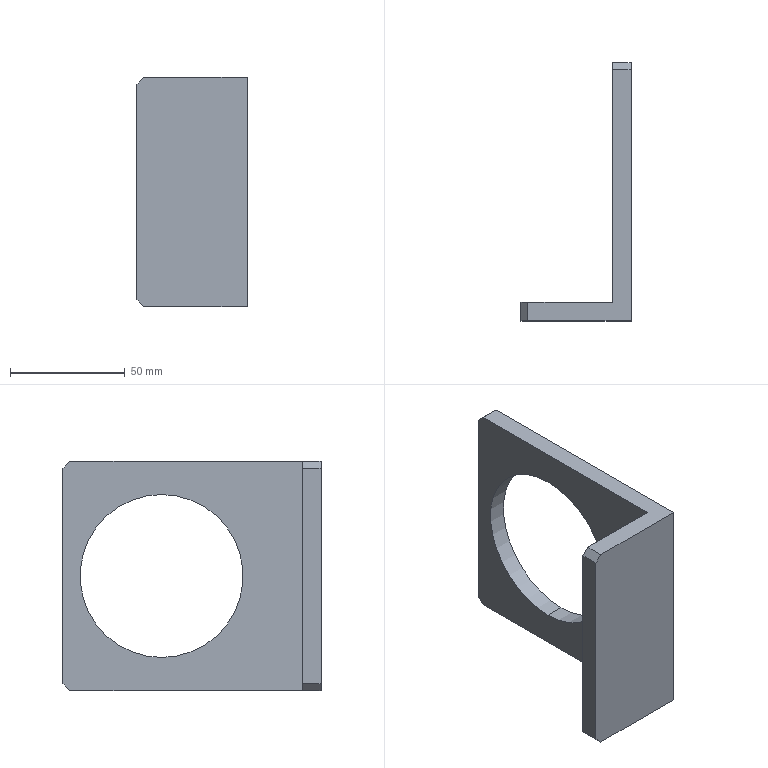Part | SolidWorks | features Chamfer 1, Extrusion 1, ICE 1 | 1 solid | 14 faces | box 48 x 112.5 x 100 mm | volume 90182 mm3 | plane 12 | cylinder 2 | commonest cylinder face diameters 71 x2
STEP:
#1=CARTESIAN_POINT('',(0.,69.5,1.121));
#2=VERTEX_POINT('',#1);
#3=CARTESIAN_POINT('',(0.,69.5,-69.879));
#4=VERTEX_POINT('',#3);
#5=CARTESIAN_POINT('',(0.,69.5,-34.379));
#6=DIRECTION('',(1.,0.,0.));
#7=DIRECTION('',(0.,0.,1.));
#8=AXIS2_PLACEMENT_3D('',#5,#6,#7);
#9=CIRCLE('',#8,35.5);
#10=EDGE_CURVE('',#2,#4,#9,.T.);
#11=ORIENTED_EDGE('',*,*,#10,.T.);
#12=CARTESIAN_POINT('',(-8.,69.5,-69.879));
#13=VERTEX_POINT('',#12);
#14=CARTESIAN_POINT('',(0.001,69.5,-69.879));
#15=DIRECTION('',(-1.,0.,0.));
#16=VECTOR('',#15,1000.);
#17=LINE('',#14,#16);
#18=EDGE_CURVE('',#4,#13,#17,.T.);
#19=ORIENTED_EDGE('',*,*,#18,.T.);
#20=CARTESIAN_POINT('',(-8.,69.5,1.121));
#21=VERTEX_POINT('',#20);
#22=CARTESIAN_POINT('',(-8.,69.5,-34.379));
#23=DIRECTION('',(-1.,0.,0.));
#24=DIRECTION('',(0.,0.,1.));
#25=AXIS2_PLACEMENT_3D('',#22,#23,#24);
#26=CIRCLE('',#25,35.5);
#27=EDGE_CURVE('',#13,#21,#26,.T.);
#28=ORIENTED_EDGE('',*,*,#27,.T.);
#29=CARTESIAN_POINT('',(0.001,69.5,1.121));
#30=DIRECTION('',(-1.,0.,0.));
#31=VECTOR('',#30,1000.);
#32=LINE('',#29,#31);
#33=EDGE_CURVE('',#2,#21,#32,.T.);
#34=ORIENTED_EDGE('',*,*,#33,.F.);
#35=EDGE_LOOP('',(#11,#19,#28,#34));
#36=FACE_OUTER_BOUND('',#35,.T.);
#37=CARTESIAN_POINT('',(0.001,69.5,-34.379));
#38=DIRECTION('',(-1.,0.,0.));
#39=DIRECTION('',(0.,0.,1.));
#40=AXIS2_PLACEMENT_3D('',#37,#38,#39);
#41=CYLINDRICAL_SURFACE('',#40,35.5);
#42=ADVANCED_FACE('',(#36),#41,.F.);
#43=CARTESIAN_POINT('',(-8.,112.5,12.621));
#44=VERTEX_POINT('',#43);
#45=CARTESIAN_POINT('',(-8.,112.5,-81.379));
#46=VERTEX_POINT('',#45);
#47=CARTESIAN_POINT('',(-8.,112.5,15.621));
#48=DIRECTION('',(0.,0.,-1.));
#49=VECTOR('',#48,1000.);
#50=LINE('',#47,#49);
#51=EDGE_CURVE('',#44,#46,#50,.T.);
#52=ORIENTED_EDGE('',*,*,#51,.F.);
#53=CARTESIAN_POINT('',(0.,112.5,12.621));
#54=VERTEX_POINT('',#53);
#55=CARTESIAN_POINT('',(-8.,112.5,12.621));
#56=DIRECTION('',(1.,0.,0.));
#57=VECTOR('',#56,1000.);
#58=LINE('',#55,#57);
#59=EDGE_CURVE('',#44,#54,#58,.T.);
#60=ORIENTED_EDGE('',*,*,#59,.T.);
#61=CARTESIAN_POINT('',(0.,112.5,-81.379));
#62=VERTEX_POINT('',#61);
#63=CARTESIAN_POINT('',(0.,112.5,15.621));
#64=DIRECTION('',(0.,0.,-1.));
#65=VECTOR('',#64,1000.);
#66=LINE('',#63,#65);
#67=EDGE_CURVE('',#54,#62,#66,.T.);
#68=ORIENTED_EDGE('',*,*,#67,.T.);
#69=CARTESIAN_POINT('',(-8.,112.5,-81.379));
#70=DIRECTION('',(-1.,0.,0.));
#71=VECTOR('',#70,1000.);
#72=LINE('',#69,#71);
#73=EDGE_CURVE('',#62,#46,#72,.T.);
#74=ORIENTED_EDGE('',*,*,#73,.T.);
#75=EDGE_LOOP('',(#52,#60,#68,#74));
#76=FACE_OUTER_BOUND('',#75,.T.);
#77=CARTESIAN_POINT('',(-8.,112.5,15.621));
#78=DIRECTION('',(0.,-1.,0.));
#79=DIRECTION('',(0.,0.,-1.));
#80=AXIS2_PLACEMENT_3D('',#77,#78,#79);
#81=PLANE('',#80);
#82=ADVANCED_FACE('',(#76),#81,.F.);
#83=CARTESIAN_POINT('',(-8.,69.5,-34.379));
#84=DIRECTION('',(-1.,0.,0.));
#85=DIRECTION('',(0.,0.,1.));
#86=AXIS2_PLACEMENT_3D('',#83,#84,#85);
#87=CIRCLE('',#86,35.5);
#88=EDGE_CURVE('',#21,#13,#87,.T.);
#89=ORIENTED_EDGE('',*,*,#88,.F.);
#90=ORIENTED_EDGE('',*,*,#27,.F.);
#91=EDGE_LOOP('',(#89,#90));
#92=FACE_BOUND('',#91,.T.);
#93=CARTESIAN_POINT('',(-8.,109.5,15.621));
#94=VERTEX_POINT('',#93);
#95=CARTESIAN_POINT('',(-8.,8.,15.621));
#96=VERTEX_POINT('',#95);
#97=CARTESIAN_POINT('',(-8.,8.,15.621));
#98=DIRECTION('',(0.,-1.,0.));
#99=VECTOR('',#98,1000.);
#100=LINE('',#97,#99);
#101=EDGE_CURVE('',#94,#96,#100,.T.);
#102=ORIENTED_EDGE('',*,*,#101,.F.);
#103=CARTESIAN_POINT('',(-8.,109.5,15.621));
#104=DIRECTION('',(0.,0.7071,-0.7071));
#105=VECTOR('',#104,1000.);
#106=LINE('',#103,#105);
#107=EDGE_CURVE('',#94,#44,#106,.T.);
#108=ORIENTED_EDGE('',*,*,#107,.T.);
#109=ORIENTED_EDGE('',*,*,#51,.T.);
#110=CARTESIAN_POINT('',(-8.,109.5,-84.379));
#111=VERTEX_POINT('',#110);
#112=CARTESIAN_POINT('',(-8.,112.5,-81.379));
#113=DIRECTION('',(0.,-0.7071,-0.7071));
#114=VECTOR('',#113,1000.);
#115=LINE('',#112,#114);
#116=EDGE_CURVE('',#46,#111,#115,.T.);
#117=ORIENTED_EDGE('',*,*,#116,.T.);
#118=CARTESIAN_POINT('',(-8.,8.,-84.379));
#119=VERTEX_POINT('',#118);
#120=CARTESIAN_POINT('',(-8.,8.,-84.379));
#121=DIRECTION('',(0.,-1.,0.));
#122=VECTOR('',#121,1000.);
#123=LINE('',#120,#122);
#124=EDGE_CURVE('',#111,#119,#123,.T.);
#125=ORIENTED_EDGE('',*,*,#124,.T.);
#126=CARTESIAN_POINT('',(-8.,8.,15.621));
#127=DIRECTION('',(0.,0.,-1.));
#128=VECTOR('',#127,1000.);
#129=LINE('',#126,#128);
#130=EDGE_CURVE('',#96,#119,#129,.T.);
#131=ORIENTED_EDGE('',*,*,#130,.F.);
#132=EDGE_LOOP('',(#102,#108,#109,#117,#125,#131));
#133=FACE_OUTER_BOUND('',#132,.T.);
#134=CARTESIAN_POINT('',(-8.,8.,15.621));
#135=DIRECTION('',(1.,0.,0.));
#136=DIRECTION('',(0.,0.,-1.));
#137=AXIS2_PLACEMENT_3D('',#134,#135,#136);
#138=PLANE('',#137);
#139=ADVANCED_FACE('',(#92,#133),#138,.F.);
#140=CARTESIAN_POINT('',(-45.,8.,-84.379));
#141=VERTEX_POINT('',#140);
#142=CARTESIAN_POINT('',(-48.,8.,-84.379));
#143=DIRECTION('',(-1.,0.,0.));
#144=VECTOR('',#143,1000.);
#145=LINE('',#142,#144);
#146=EDGE_CURVE('',#119,#141,#145,.T.);
#147=ORIENTED_EDGE('',*,*,#146,.T.);
#148=CARTESIAN_POINT('',(-48.,8.,-81.379));
#149=VERTEX_POINT('',#148);
#150=CARTESIAN_POINT('',(-48.,8.,-81.379));
#151=DIRECTION('',(-0.7071,0.,0.7071));
#152=VECTOR('',#151,1000.);
#153=LINE('',#150,#152);
#154=EDGE_CURVE('',#141,#149,#153,.T.);
#155=ORIENTED_EDGE('',*,*,#154,.T.);
#156=CARTESIAN_POINT('',(-48.,8.,12.621));
#157=VERTEX_POINT('',#156);
#158=CARTESIAN_POINT('',(-48.,8.,15.621));
#159=DIRECTION('',(0.,0.,-1.));
#160=VECTOR('',#159,1000.);
#161=LINE('',#158,#160);
#162=EDGE_CURVE('',#157,#149,#161,.T.);
#163=ORIENTED_EDGE('',*,*,#162,.F.);
#164=CARTESIAN_POINT('',(-45.,8.,15.621));
#165=VERTEX_POINT('',#164);
#166=CARTESIAN_POINT('',(-45.,8.,15.621));
#167=DIRECTION('',(0.7071,0.,0.7071));
#168=VECTOR('',#167,1000.);
#169=LINE('',#166,#168);
#170=EDGE_CURVE('',#157,#165,#169,.T.);
#171=ORIENTED_EDGE('',*,*,#170,.T.);
#172=CARTESIAN_POINT('',(-48.,8.,15.621));
#173=DIRECTION('',(-1.,0.,0.));
#174=VECTOR('',#173,1000.);
#175=LINE('',#172,#174);
#176=EDGE_CURVE('',#96,#165,#175,.T.);
#177=ORIENTED_EDGE('',*,*,#176,.F.);
#178=ORIENTED_EDGE('',*,*,#130,.T.);
#179=EDGE_LOOP('',(#147,#155,#163,#171,#177,#178));
#180=FACE_OUTER_BOUND('',#179,.T.);
#181=CARTESIAN_POINT('',(-48.,8.,15.621));
#182=DIRECTION('',(0.,-1.,0.));
#183=DIRECTION('',(1.,0.,0.));
#184=AXIS2_PLACEMENT_3D('',#181,#182,#183);
#185=PLANE('',#184);
#186=ADVANCED_FACE('',(#180),#185,.F.);
#187=ORIENTED_EDGE('',*,*,#162,.T.);
#188=CARTESIAN_POINT('',(-48.,0.,-81.379));
#189=VERTEX_POINT('',#188);
#190=CARTESIAN_POINT('',(-48.,0.,-81.379));
#191=DIRECTION('',(0.,-1.,0.));
#192=VECTOR('',#191,1000.);
#193=LINE('',#190,#192);
#194=EDGE_CURVE('',#149,#189,#193,.T.);
#195=ORIENTED_EDGE('',*,*,#194,.T.);
#196=CARTESIAN_POINT('',(-48.,0.,12.621));
#197=VERTEX_POINT('',#196);
#198=CARTESIAN_POINT('',(-48.,0.,15.621));
#199=DIRECTION('',(0.,0.,-1.));
#200=VECTOR('',#199,1000.);
#201=LINE('',#198,#200);
#202=EDGE_CURVE('',#197,#189,#201,.T.);
#203=ORIENTED_EDGE('',*,*,#202,.F.);
#204=CARTESIAN_POINT('',(-48.,0.,12.621));
#205=DIRECTION('',(0.,1.,0.));
#206=VECTOR('',#205,1000.);
#207=LINE('',#204,#206);
#208=EDGE_CURVE('',#197,#157,#207,.T.);
#209=ORIENTED_EDGE('',*,*,#208,.T.);
#210=EDGE_LOOP('',(#187,#195,#203,#209));
#211=FACE_OUTER_BOUND('',#210,.T.);
#212=CARTESIAN_POINT('',(-48.,0.,15.621));
#213=DIRECTION('',(1.,0.,0.));
#214=DIRECTION('',(0.,0.,-1.));
#215=AXIS2_PLACEMENT_3D('',#212,#213,#214);
#216=PLANE('',#215);
#217=ADVANCED_FACE('',(#211),#216,.F.);
#218=ORIENTED_EDGE('',*,*,#202,.T.);
#219=CARTESIAN_POINT('',(-45.,0.,-84.379));
#220=VERTEX_POINT('',#219);
#221=CARTESIAN_POINT('',(-48.,0.,-81.379));
#222=DIRECTION('',(0.7071,0.,-0.7071));
#223=VECTOR('',#222,1000.);
#224=LINE('',#221,#223);
#225=EDGE_CURVE('',#189,#220,#224,.T.);
#226=ORIENTED_EDGE('',*,*,#225,.T.);
#227=CARTESIAN_POINT('',(0.,0.,-84.379));
#228=VERTEX_POINT('',#227);
#229=CARTESIAN_POINT('',(0.,0.,-84.379));
#230=DIRECTION('',(1.,0.,0.));
#231=VECTOR('',#230,1000.);
#232=LINE('',#229,#231);
#233=EDGE_CURVE('',#220,#228,#232,.T.);
#234=ORIENTED_EDGE('',*,*,#233,.T.);
#235=CARTESIAN_POINT('',(0.,0.,15.621));
#236=VERTEX_POINT('',#235);
#237=CARTESIAN_POINT('',(0.,0.,15.621));
#238=DIRECTION('',(0.,0.,-1.));
#239=VECTOR('',#238,1000.);
#240=LINE('',#237,#239);
#241=EDGE_CURVE('',#236,#228,#240,.T.);
#242=ORIENTED_EDGE('',*,*,#241,.F.);
#243=CARTESIAN_POINT('',(-45.,0.,15.621));
#244=VERTEX_POINT('',#243);
#245=CARTESIAN_POINT('',(0.,0.,15.621));
#246=DIRECTION('',(1.,0.,0.));
#247=VECTOR('',#246,1000.);
#248=LINE('',#245,#247);
#249=EDGE_CURVE('',#244,#236,#248,.T.);
#250=ORIENTED_EDGE('',*,*,#249,.F.);
#251=CARTESIAN_POINT('',(-45.,0.,15.621));
#252=DIRECTION('',(-0.7071,0.,-0.7071));
#253=VECTOR('',#252,1000.);
#254=LINE('',#251,#253);
#255=EDGE_CURVE('',#244,#197,#254,.T.);
#256=ORIENTED_EDGE('',*,*,#255,.T.);
#257=EDGE_LOOP('',(#218,#226,#234,#242,#250,#256));
#258=FACE_OUTER_BOUND('',#257,.T.);
#259=CARTESIAN_POINT('',(0.,0.,15.621));
#260=DIRECTION('',(0.,1.,0.));
#261=DIRECTION('',(-1.,0.,0.));
#262=AXIS2_PLACEMENT_3D('',#259,#260,#261);
#263=PLANE('',#262);
#264=ADVANCED_FACE('',(#258),#263,.F.);
#265=ORIENTED_EDGE('',*,*,#10,.F.);
#266=CARTESIAN_POINT('',(0.,69.5,-34.379));
#267=DIRECTION('',(1.,0.,0.));
#268=DIRECTION('',(0.,0.,1.));
#269=AXIS2_PLACEMENT_3D('',#266,#267,#268);
#270=CIRCLE('',#269,35.5);
#271=EDGE_CURVE('',#4,#2,#270,.T.);
#272=ORIENTED_EDGE('',*,*,#271,.F.);
#273=EDGE_LOOP('',(#265,#272));
#274=FACE_BOUND('',#273,.T.);
#275=ORIENTED_EDGE('',*,*,#67,.F.);
#276=CARTESIAN_POINT('',(0.,109.5,15.621));
#277=VERTEX_POINT('',#276);
#278=CARTESIAN_POINT('',(0.,109.5,15.621));
#279=DIRECTION('',(0.,-0.7071,0.7071));
#280=VECTOR('',#279,1000.);
#281=LINE('',#278,#280);
#282=EDGE_CURVE('',#54,#277,#281,.T.);
#283=ORIENTED_EDGE('',*,*,#282,.T.);
#284=CARTESIAN_POINT('',(0.,112.5,15.621));
#285=DIRECTION('',(0.,1.,0.));
#286=VECTOR('',#285,1000.);
#287=LINE('',#284,#286);
#288=EDGE_CURVE('',#236,#277,#287,.T.);
#289=ORIENTED_EDGE('',*,*,#288,.F.);
#290=ORIENTED_EDGE('',*,*,#241,.T.);
#291=CARTESIAN_POINT('',(0.,109.5,-84.379));
#292=VERTEX_POINT('',#291);
#293=CARTESIAN_POINT('',(0.,112.5,-84.379));
#294=DIRECTION('',(0.,1.,0.));
#295=VECTOR('',#294,1000.);
#296=LINE('',#293,#295);
#297=EDGE_CURVE('',#228,#292,#296,.T.);
#298=ORIENTED_EDGE('',*,*,#297,.T.);
#299=CARTESIAN_POINT('',(0.,112.5,-81.379));
#300=DIRECTION('',(0.,0.7071,0.7071));
#301=VECTOR('',#300,1000.);
#302=LINE('',#299,#301);
#303=EDGE_CURVE('',#292,#62,#302,.T.);
#304=ORIENTED_EDGE('',*,*,#303,.T.);
#305=EDGE_LOOP('',(#275,#283,#289,#290,#298,#304));
#306=FACE_OUTER_BOUND('',#305,.T.);
#307=CARTESIAN_POINT('',(0.,112.5,15.621));
#308=DIRECTION('',(-1.,0.,0.));
#309=DIRECTION('',(0.,0.,1.));
#310=AXIS2_PLACEMENT_3D('',#307,#308,#309);
#311=PLANE('',#310);
#312=ADVANCED_FACE('',(#274,#306),#311,.F.);
#313=ORIENTED_EDGE('',*,*,#176,.T.);
#314=CARTESIAN_POINT('',(-45.,0.,15.621));
#315=DIRECTION('',(0.,-1.,0.));
#316=VECTOR('',#315,1000.);
#317=LINE('',#314,#316);
#318=EDGE_CURVE('',#165,#244,#317,.T.);
#319=ORIENTED_EDGE('',*,*,#318,.T.);
#320=ORIENTED_EDGE('',*,*,#249,.T.);
#321=ORIENTED_EDGE('',*,*,#288,.T.);
#322=CARTESIAN_POINT('',(0.,109.5,15.621));
#323=DIRECTION('',(-1.,0.,0.));
#324=VECTOR('',#323,1000.);
#325=LINE('',#322,#324);
#326=EDGE_CURVE('',#277,#94,#325,.T.);
#327=ORIENTED_EDGE('',*,*,#326,.T.);
#328=ORIENTED_EDGE('',*,*,#101,.T.);
#329=EDGE_LOOP('',(#313,#319,#320,#321,#327,#328));
#330=FACE_OUTER_BOUND('',#329,.T.);
#331=CARTESIAN_POINT('',(0.,0.,15.621));
#332=DIRECTION('',(0.,0.,-1.));
#333=DIRECTION('',(-1.,0.,0.));
#334=AXIS2_PLACEMENT_3D('',#331,#332,#333);
#335=PLANE('',#334);
#336=ADVANCED_FACE('',(#330),#335,.F.);
#337=ORIENTED_EDGE('',*,*,#233,.F.);
#338=CARTESIAN_POINT('',(-45.,8.,-84.379));
#339=DIRECTION('',(0.,1.,0.));
#340=VECTOR('',#339,1000.);
#341=LINE('',#338,#340);
#342=EDGE_CURVE('',#220,#141,#341,.T.);
#343=ORIENTED_EDGE('',*,*,#342,.T.);
#344=ORIENTED_EDGE('',*,*,#146,.F.);
#345=ORIENTED_EDGE('',*,*,#124,.F.);
#346=CARTESIAN_POINT('',(0.,109.5,-84.379));
#347=DIRECTION('',(1.,0.,0.));
#348=VECTOR('',#347,1000.);
#349=LINE('',#346,#348);
#350=EDGE_CURVE('',#111,#292,#349,.T.);
#351=ORIENTED_EDGE('',*,*,#350,.T.);
#352=ORIENTED_EDGE('',*,*,#297,.F.);
#353=EDGE_LOOP('',(#337,#343,#344,#345,#351,#352));
#354=FACE_OUTER_BOUND('',#353,.T.);
#355=CARTESIAN_POINT('',(0.,0.,-84.379));
#356=DIRECTION('',(0.,0.,-1.));
#357=DIRECTION('',(-1.,0.,0.));
#358=AXIS2_PLACEMENT_3D('',#355,#356,#357);
#359=PLANE('',#358);
#360=ADVANCED_FACE('',(#354),#359,.T.);
#361=ORIENTED_EDGE('',*,*,#154,.F.);
#362=ORIENTED_EDGE('',*,*,#342,.F.);
#363=ORIENTED_EDGE('',*,*,#225,.F.);
#364=ORIENTED_EDGE('',*,*,#194,.F.);
#365=EDGE_LOOP('',(#361,#362,#363,#364));
#366=FACE_OUTER_BOUND('',#365,.T.);
#367=CARTESIAN_POINT('',(-48.,0.,-81.379));
#368=DIRECTION('',(-0.7071,0.,-0.7071));
#369=DIRECTION('',(0.,1.,0.));
#370=AXIS2_PLACEMENT_3D('',#367,#368,#369);
#371=PLANE('',#370);
#372=ADVANCED_FACE('',(#366),#371,.T.);
#373=ORIENTED_EDGE('',*,*,#170,.F.);
#374=ORIENTED_EDGE('',*,*,#208,.F.);
#375=ORIENTED_EDGE('',*,*,#255,.F.);
#376=ORIENTED_EDGE('',*,*,#318,.F.);
#377=EDGE_LOOP('',(#373,#374,#375,#376));
#378=FACE_OUTER_BOUND('',#377,.T.);
#379=CARTESIAN_POINT('',(-45.,0.,15.621));
#380=DIRECTION('',(0.7071,0.,-0.7071));
#381=DIRECTION('',(0.,-1.,0.));
#382=AXIS2_PLACEMENT_3D('',#379,#380,#381);
#383=PLANE('',#382);
#384=ADVANCED_FACE('',(#378),#383,.F.);
#385=ORIENTED_EDGE('',*,*,#282,.F.);
#386=ORIENTED_EDGE('',*,*,#59,.F.);
#387=ORIENTED_EDGE('',*,*,#107,.F.);
#388=ORIENTED_EDGE('',*,*,#326,.F.);
#389=EDGE_LOOP('',(#385,#386,#387,#388));
#390=FACE_OUTER_BOUND('',#389,.T.);
#391=CARTESIAN_POINT('',(0.,109.5,15.621));
#392=DIRECTION('',(0.,-0.7071,-0.7071));
#393=DIRECTION('',(-1.,0.,0.));
#394=AXIS2_PLACEMENT_3D('',#391,#392,#393);
#395=PLANE('',#394);
#396=ADVANCED_FACE('',(#390),#395,.F.);
#397=ORIENTED_EDGE('',*,*,#303,.F.);
#398=ORIENTED_EDGE('',*,*,#350,.F.);
#399=ORIENTED_EDGE('',*,*,#116,.F.);
#400=ORIENTED_EDGE('',*,*,#73,.F.);
#401=EDGE_LOOP('',(#397,#398,#399,#400));
#402=FACE_OUTER_BOUND('',#401,.T.);
#403=CARTESIAN_POINT('',(-8.,112.5,-81.379));
#404=DIRECTION('',(0.,0.7071,-0.7071));
#405=DIRECTION('',(1.,0.,0.));
#406=AXIS2_PLACEMENT_3D('',#403,#404,#405);
#407=PLANE('',#406);
#408=ADVANCED_FACE('',(#402),#407,.T.);
#409=ORIENTED_EDGE('',*,*,#18,.F.);
#410=ORIENTED_EDGE('',*,*,#271,.T.);
#411=ORIENTED_EDGE('',*,*,#33,.T.);
#412=ORIENTED_EDGE('',*,*,#88,.T.);
#413=EDGE_LOOP('',(#409,#410,#411,#412));
#414=FACE_OUTER_BOUND('',#413,.T.);
#415=CARTESIAN_POINT('',(0.001,69.5,-34.379));
#416=DIRECTION('',(-1.,0.,0.));
#417=DIRECTION('',(0.,0.,1.));
#418=AXIS2_PLACEMENT_3D('',#415,#416,#417);
#419=CYLINDRICAL_SURFACE('',#418,35.5);
#420=ADVANCED_FACE('',(#414),#419,.F.);
#421=CLOSED_SHELL('',(#42,#82,#139,#186,#217,#264,#312,#336,#360,#372,#384,#396,#408,#420));
#422=MANIFOLD_SOLID_BREP('',#421);
#423=CARTESIAN_POINT('',(0.,0.,0.));
#424=DIRECTION('',(0.,0.,1.));
#425=DIRECTION('',(1.,0.,0.));
#426=AXIS2_PLACEMENT_3D('',#423,#424,#425);
#427=(LENGTH_UNIT()NAMED_UNIT(*)SI_UNIT(.MILLI.,.METRE.));
#428=UNCERTAINTY_MEASURE_WITH_UNIT(LENGTH_MEASURE(0.00001),#427,'','');
#429=(NAMED_UNIT(*)PLANE_ANGLE_UNIT()SI_UNIT($,.RADIAN.));
#430=(NAMED_UNIT(*)SI_UNIT($,.STERADIAN.)SOLID_ANGLE_UNIT());
#431=(GEOMETRIC_REPRESENTATION_CONTEXT(3)GLOBAL_UNCERTAINTY_ASSIGNED_CONTEXT((#428))GLOBAL_UNIT_ASSIGNED_CONTEXT((#427,#429,#430))REPRESENTATION_CONTEXT('',''));
#432=ADVANCED_BREP_SHAPE_REPRESENTATION('',(#422,#426),#431);